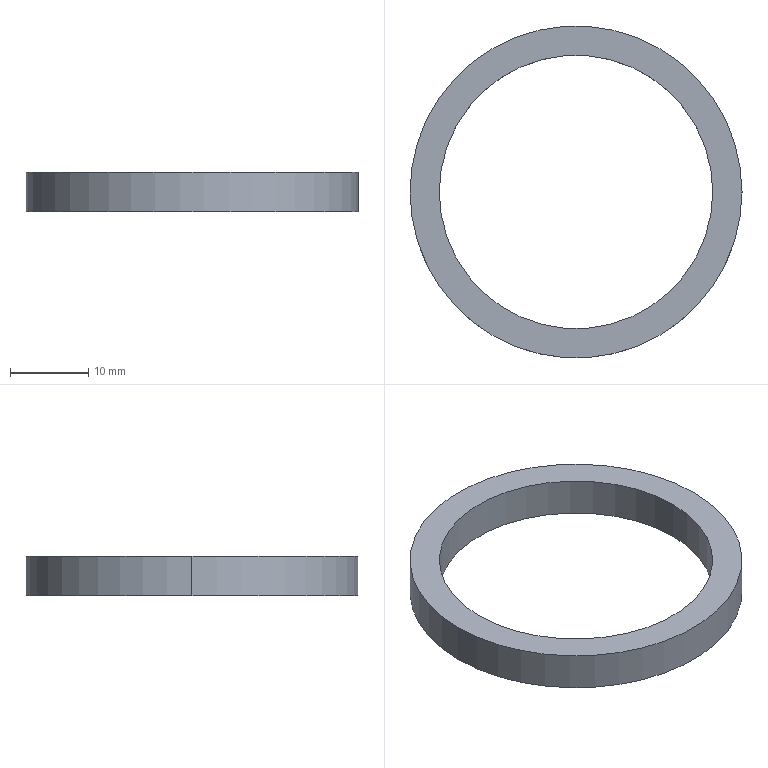Part | SolidWorks | features Extrusion 1 | 1 solid | 6 faces | box 42.5 x 42.5 x 5 mm | volume 2283 mm3 | cylinder 4 | plane 2 | commonest cylinder face diameters 35 x2 42.5 x2
STEP:
#1=CARTESIAN_POINT('',(-17.5,0.,5.));
#2=VERTEX_POINT('',#1);
#3=CARTESIAN_POINT('',(17.5,0.,5.));
#4=VERTEX_POINT('',#3);
#5=CARTESIAN_POINT('',(0.,0.,5.));
#6=DIRECTION('',(0.,0.,1.));
#7=DIRECTION('',(1.,0.,0.));
#8=AXIS2_PLACEMENT_3D('',#5,#6,#7);
#9=CIRCLE('',#8,17.5);
#10=EDGE_CURVE('',#2,#4,#9,.T.);
#11=ORIENTED_EDGE('',*,*,#10,.T.);
#12=CARTESIAN_POINT('',(17.5,0.,0.));
#13=VERTEX_POINT('',#12);
#14=CARTESIAN_POINT('',(17.5,0.,5.));
#15=DIRECTION('',(0.,0.,-1.));
#16=VECTOR('',#15,1000.);
#17=LINE('',#14,#16);
#18=EDGE_CURVE('',#4,#13,#17,.T.);
#19=ORIENTED_EDGE('',*,*,#18,.T.);
#20=CARTESIAN_POINT('',(-17.5,0.,0.));
#21=VERTEX_POINT('',#20);
#22=CARTESIAN_POINT('',(0.,0.,0.));
#23=DIRECTION('',(0.,0.,1.));
#24=DIRECTION('',(1.,0.,0.));
#25=AXIS2_PLACEMENT_3D('',#22,#23,#24);
#26=CIRCLE('',#25,17.5);
#27=EDGE_CURVE('',#21,#13,#26,.T.);
#28=ORIENTED_EDGE('',*,*,#27,.F.);
#29=CARTESIAN_POINT('',(-17.5,0.,5.));
#30=DIRECTION('',(0.,0.,-1.));
#31=VECTOR('',#30,1000.);
#32=LINE('',#29,#31);
#33=EDGE_CURVE('',#2,#21,#32,.T.);
#34=ORIENTED_EDGE('',*,*,#33,.F.);
#35=EDGE_LOOP('',(#11,#19,#28,#34));
#36=FACE_OUTER_BOUND('',#35,.T.);
#37=CARTESIAN_POINT('',(0.,0.,5.));
#38=DIRECTION('',(0.,0.,-1.));
#39=DIRECTION('',(-1.,0.,0.));
#40=AXIS2_PLACEMENT_3D('',#37,#38,#39);
#41=CYLINDRICAL_SURFACE('',#40,17.5);
#42=ADVANCED_FACE('',(#36),#41,.F.);
#43=CARTESIAN_POINT('',(21.25,0.,5.));
#44=VERTEX_POINT('',#43);
#45=CARTESIAN_POINT('',(-21.25,0.,5.));
#46=VERTEX_POINT('',#45);
#47=CARTESIAN_POINT('',(0.,0.,5.));
#48=DIRECTION('',(0.,0.,1.));
#49=DIRECTION('',(1.,0.,0.));
#50=AXIS2_PLACEMENT_3D('',#47,#48,#49);
#51=CIRCLE('',#50,21.25);
#52=EDGE_CURVE('',#44,#46,#51,.T.);
#53=ORIENTED_EDGE('',*,*,#52,.F.);
#54=CARTESIAN_POINT('',(21.25,0.,0.));
#55=VERTEX_POINT('',#54);
#56=CARTESIAN_POINT('',(21.25,0.,5.));
#57=DIRECTION('',(0.,0.,-1.));
#58=VECTOR('',#57,1000.);
#59=LINE('',#56,#58);
#60=EDGE_CURVE('',#44,#55,#59,.T.);
#61=ORIENTED_EDGE('',*,*,#60,.T.);
#62=CARTESIAN_POINT('',(-21.25,0.,0.));
#63=VERTEX_POINT('',#62);
#64=CARTESIAN_POINT('',(0.,0.,0.));
#65=DIRECTION('',(0.,0.,1.));
#66=DIRECTION('',(1.,0.,0.));
#67=AXIS2_PLACEMENT_3D('',#64,#65,#66);
#68=CIRCLE('',#67,21.25);
#69=EDGE_CURVE('',#55,#63,#68,.T.);
#70=ORIENTED_EDGE('',*,*,#69,.T.);
#71=CARTESIAN_POINT('',(-21.25,0.,5.));
#72=DIRECTION('',(0.,0.,-1.));
#73=VECTOR('',#72,1000.);
#74=LINE('',#71,#73);
#75=EDGE_CURVE('',#46,#63,#74,.T.);
#76=ORIENTED_EDGE('',*,*,#75,.F.);
#77=EDGE_LOOP('',(#53,#61,#70,#76));
#78=FACE_OUTER_BOUND('',#77,.T.);
#79=CARTESIAN_POINT('',(0.,0.,5.));
#80=DIRECTION('',(0.,0.,-1.));
#81=DIRECTION('',(-1.,0.,0.));
#82=AXIS2_PLACEMENT_3D('',#79,#80,#81);
#83=CYLINDRICAL_SURFACE('',#82,21.25);
#84=ADVANCED_FACE('',(#78),#83,.T.);
#85=CARTESIAN_POINT('',(0.,0.,5.));
#86=DIRECTION('',(0.,0.,1.));
#87=DIRECTION('',(1.,0.,0.));
#88=AXIS2_PLACEMENT_3D('',#85,#86,#87);
#89=CIRCLE('',#88,21.25);
#90=EDGE_CURVE('',#46,#44,#89,.T.);
#91=ORIENTED_EDGE('',*,*,#90,.T.);
#92=ORIENTED_EDGE('',*,*,#52,.T.);
#93=EDGE_LOOP('',(#91,#92));
#94=FACE_OUTER_BOUND('',#93,.T.);
#95=ORIENTED_EDGE('',*,*,#10,.F.);
#96=CARTESIAN_POINT('',(0.,0.,5.));
#97=DIRECTION('',(0.,0.,1.));
#98=DIRECTION('',(1.,0.,0.));
#99=AXIS2_PLACEMENT_3D('',#96,#97,#98);
#100=CIRCLE('',#99,17.5);
#101=EDGE_CURVE('',#4,#2,#100,.T.);
#102=ORIENTED_EDGE('',*,*,#101,.F.);
#103=EDGE_LOOP('',(#95,#102));
#104=FACE_BOUND('',#103,.T.);
#105=CARTESIAN_POINT('',(0.,0.,5.));
#106=DIRECTION('',(0.,0.,1.));
#107=DIRECTION('',(1.,0.,0.));
#108=AXIS2_PLACEMENT_3D('',#105,#106,#107);
#109=PLANE('',#108);
#110=ADVANCED_FACE('',(#94,#104),#109,.T.);
#111=CARTESIAN_POINT('',(0.,0.,0.));
#112=DIRECTION('',(0.,0.,1.));
#113=DIRECTION('',(1.,0.,0.));
#114=AXIS2_PLACEMENT_3D('',#111,#112,#113);
#115=CIRCLE('',#114,21.25);
#116=EDGE_CURVE('',#63,#55,#115,.T.);
#117=ORIENTED_EDGE('',*,*,#116,.F.);
#118=ORIENTED_EDGE('',*,*,#69,.F.);
#119=EDGE_LOOP('',(#117,#118));
#120=FACE_OUTER_BOUND('',#119,.T.);
#121=ORIENTED_EDGE('',*,*,#27,.T.);
#122=CARTESIAN_POINT('',(0.,0.,0.));
#123=DIRECTION('',(0.,0.,1.));
#124=DIRECTION('',(1.,0.,0.));
#125=AXIS2_PLACEMENT_3D('',#122,#123,#124);
#126=CIRCLE('',#125,17.5);
#127=EDGE_CURVE('',#13,#21,#126,.T.);
#128=ORIENTED_EDGE('',*,*,#127,.T.);
#129=EDGE_LOOP('',(#121,#128));
#130=FACE_BOUND('',#129,.T.);
#131=CARTESIAN_POINT('',(0.,0.,0.));
#132=DIRECTION('',(0.,0.,1.));
#133=DIRECTION('',(1.,0.,0.));
#134=AXIS2_PLACEMENT_3D('',#131,#132,#133);
#135=PLANE('',#134);
#136=ADVANCED_FACE('',(#120,#130),#135,.F.);
#137=ORIENTED_EDGE('',*,*,#60,.F.);
#138=ORIENTED_EDGE('',*,*,#90,.F.);
#139=ORIENTED_EDGE('',*,*,#75,.T.);
#140=ORIENTED_EDGE('',*,*,#116,.T.);
#141=EDGE_LOOP('',(#137,#138,#139,#140));
#142=FACE_OUTER_BOUND('',#141,.T.);
#143=CARTESIAN_POINT('',(0.,0.,5.));
#144=DIRECTION('',(0.,0.,-1.));
#145=DIRECTION('',(-1.,0.,0.));
#146=AXIS2_PLACEMENT_3D('',#143,#144,#145);
#147=CYLINDRICAL_SURFACE('',#146,21.25);
#148=ADVANCED_FACE('',(#142),#147,.T.);
#149=ORIENTED_EDGE('',*,*,#18,.F.);
#150=ORIENTED_EDGE('',*,*,#101,.T.);
#151=ORIENTED_EDGE('',*,*,#33,.T.);
#152=ORIENTED_EDGE('',*,*,#127,.F.);
#153=EDGE_LOOP('',(#149,#150,#151,#152));
#154=FACE_OUTER_BOUND('',#153,.T.);
#155=CARTESIAN_POINT('',(0.,0.,5.));
#156=DIRECTION('',(0.,0.,-1.));
#157=DIRECTION('',(-1.,0.,0.));
#158=AXIS2_PLACEMENT_3D('',#155,#156,#157);
#159=CYLINDRICAL_SURFACE('',#158,17.5);
#160=ADVANCED_FACE('',(#154),#159,.F.);
#161=CLOSED_SHELL('',(#42,#84,#110,#136,#148,#160));
#162=MANIFOLD_SOLID_BREP('',#161);
#163=CARTESIAN_POINT('',(0.,0.,0.));
#164=DIRECTION('',(0.,0.,1.));
#165=DIRECTION('',(1.,0.,0.));
#166=AXIS2_PLACEMENT_3D('',#163,#164,#165);
#167=(LENGTH_UNIT()NAMED_UNIT(*)SI_UNIT(.MILLI.,.METRE.));
#168=UNCERTAINTY_MEASURE_WITH_UNIT(LENGTH_MEASURE(0.00001),#167,'','');
#169=(NAMED_UNIT(*)PLANE_ANGLE_UNIT()SI_UNIT($,.RADIAN.));
#170=(NAMED_UNIT(*)SI_UNIT($,.STERADIAN.)SOLID_ANGLE_UNIT());
#171=(GEOMETRIC_REPRESENTATION_CONTEXT(3)GLOBAL_UNCERTAINTY_ASSIGNED_CONTEXT((#168))GLOBAL_UNIT_ASSIGNED_CONTEXT((#167,#169,#170))REPRESENTATION_CONTEXT('',''));
#172=ADVANCED_BREP_SHAPE_REPRESENTATION('',(#162,#166),#171);